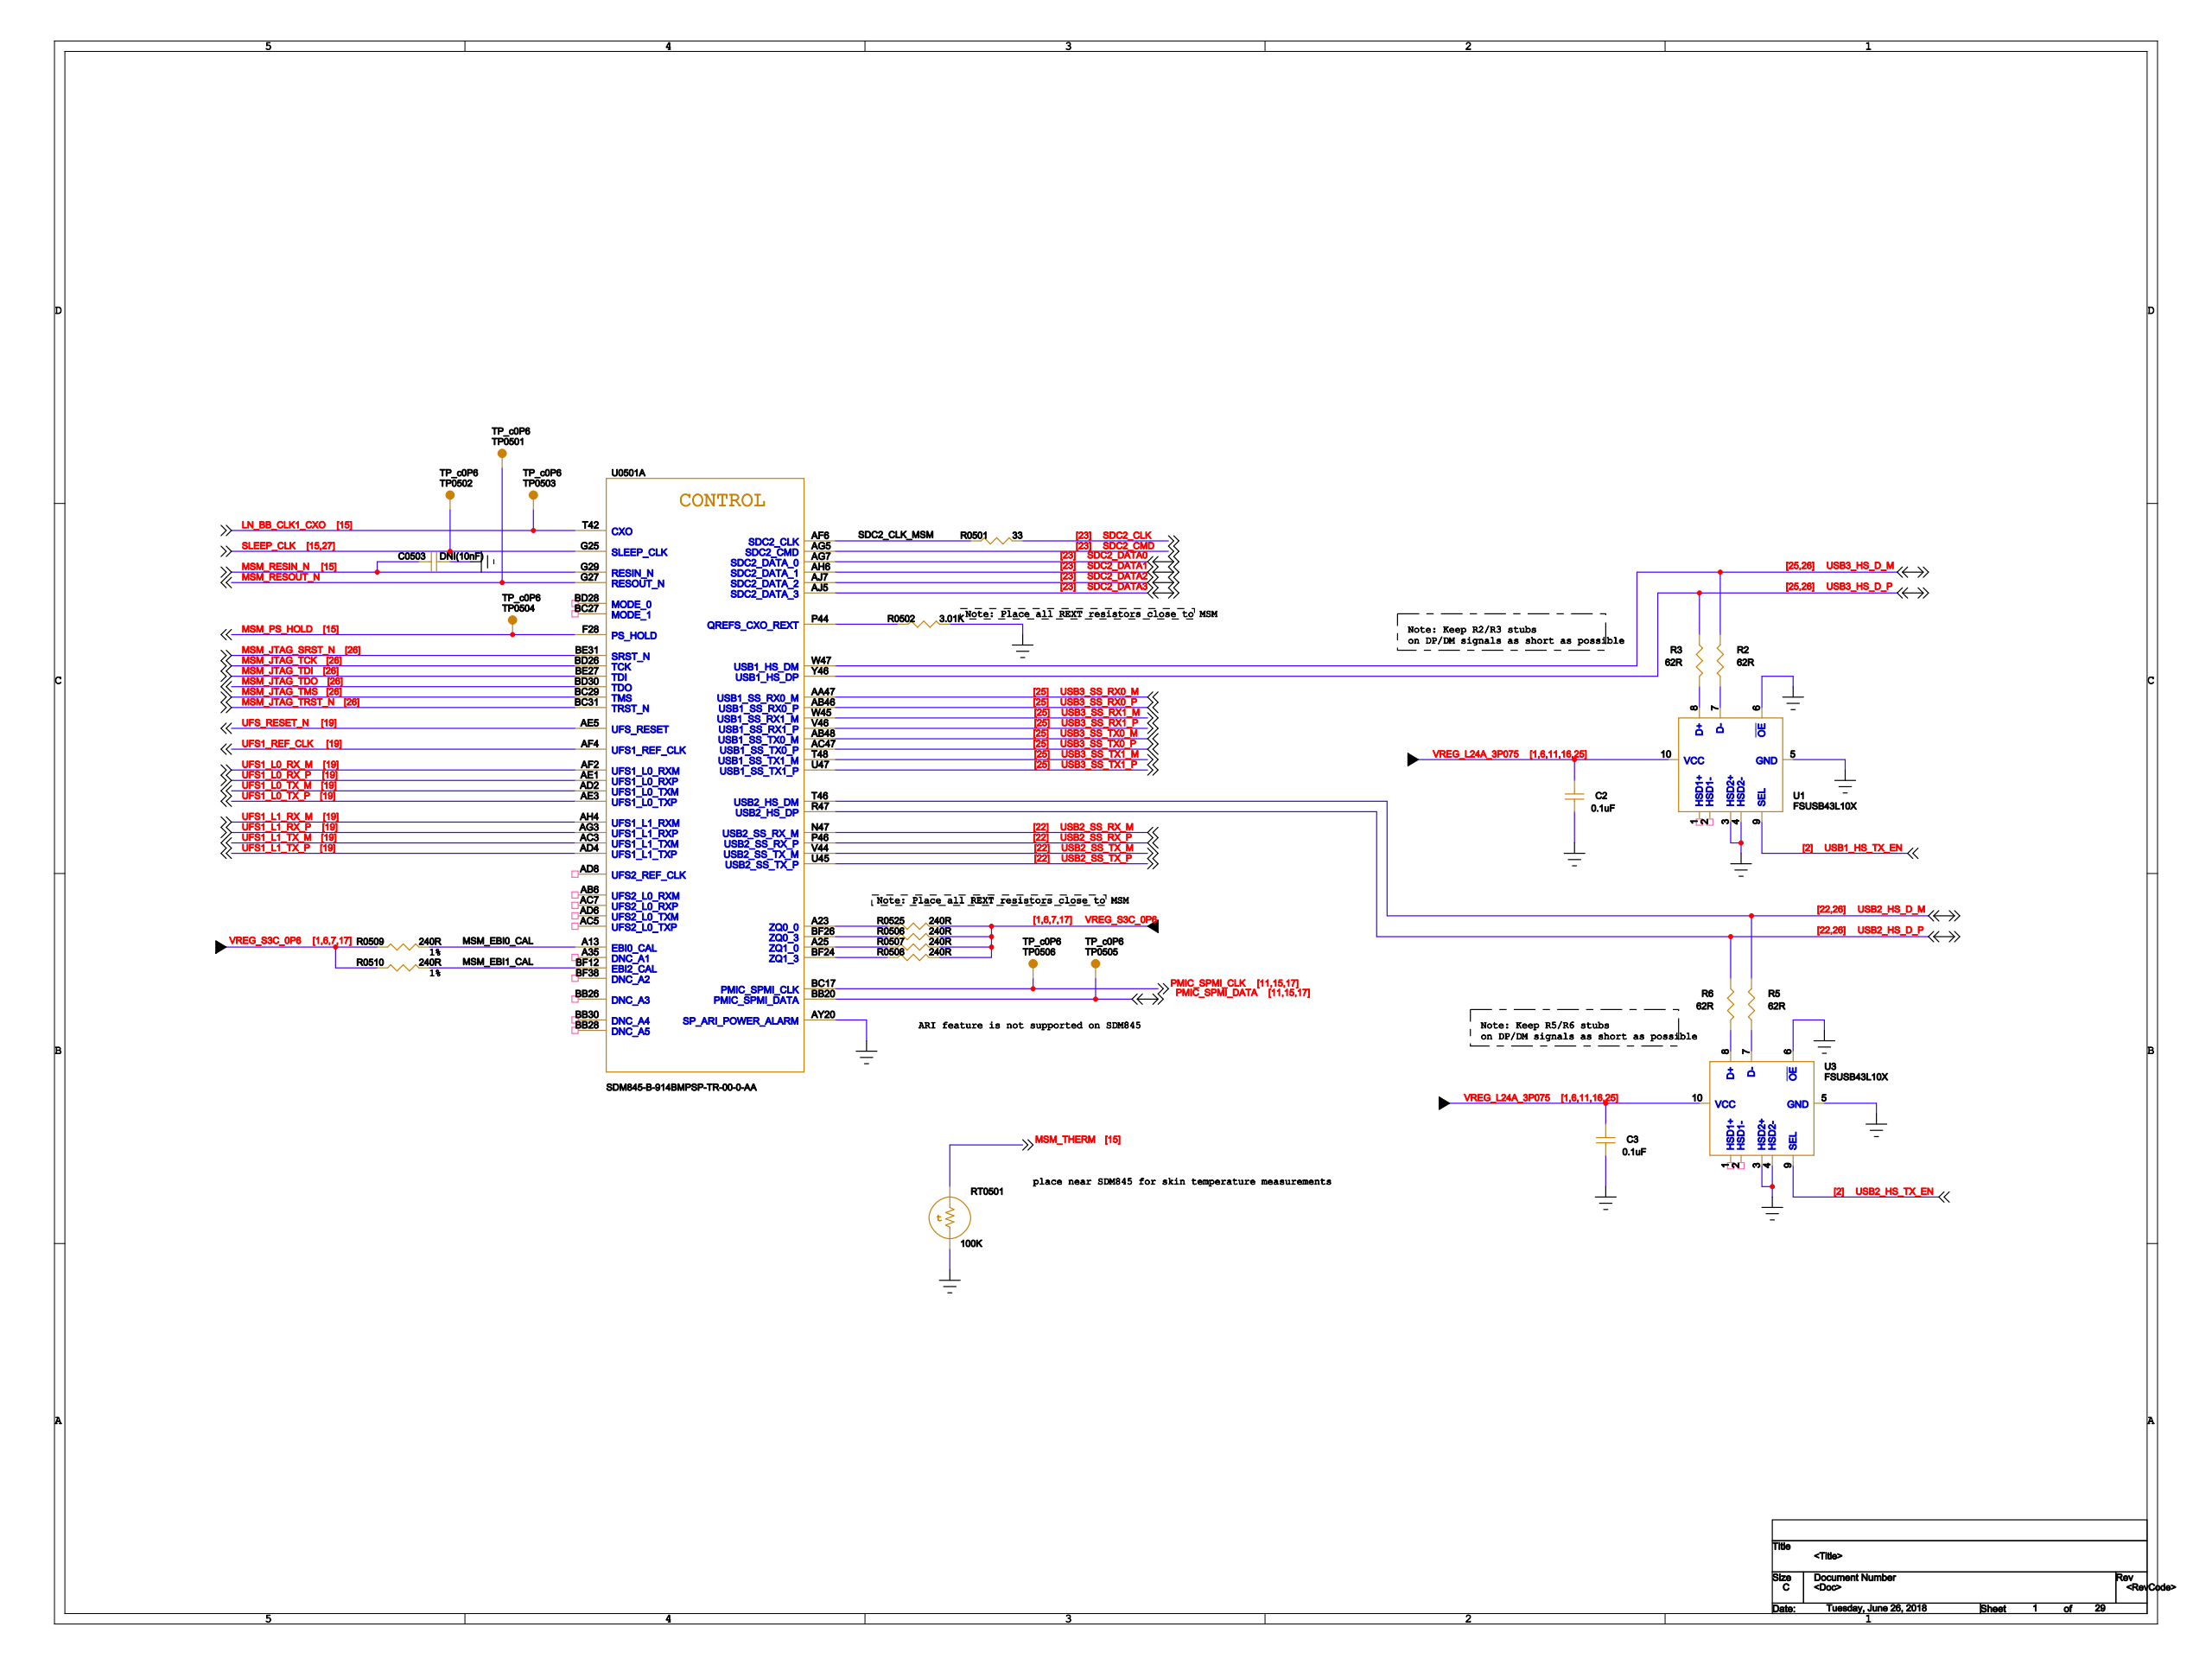Circuit board | Cadence Allegro | 802 parts | 566 nets | one sheet of the schematic
Parts on this sheet (reference | value | footprint):
C2 | 0.1uF | C0402
C3 | 0.1uF | C0402
C0503 | DNI(10nF) | C0201
R2 | 62R | R0201
R3 | 62R | R0201
R5 | 62R | R0201
R6 | 62R | R0201
R0501 | 33 | R0201
R0502 | 3.01K | R0402
R0506 | 240R | R0201
R0507 | 240R | R0201
R0508 | 240R | R0201
R0509 | 240R | R0201
R0510 | 240R | R0201
R0525 | 240R | R0201
RT0501 | 100K | R0402
TP0501 | TP_c0P6 | TP_C0P6
TP0502 | TP_c0P6 | TP_C0P6
TP0503 | TP_c0P6 | TP_C0P6
TP0504 | TP_c0P6 | TP_C0P6
TP0505 | TP_c0P6 | TP_C0P6
TP0506 | TP_c0P6 | TP_C0P6
U1 | FSUSB43L10X | UQFN10_1P6X2P1X0P5_0P65
U3 | FSUSB43L10X | UQFN10_1P6X2P1X0P5_0P65
U0501 | SDM845-B-914BMPSP-TR-00-0-AA | BGA914_12P4X12P4_0P58_0P35
Nets of these parts (net: part-pin ...):
MSM_RESIN_N: C0503-1 U0501-G29
GND: C2-1 C3-1 C0503-2 R0502-2 RT0501-2 U1-3 U1-4 U1-5 U1-6 U3-3 U3-4 U3-5 U3-6 U0501-AY20 U0501-C3 U0501-R5
VREG_L24A_3P075: C2-2 C3-2 U1-10 U3-10
SDC2_DATA3: U0501-AJ5
SDC2_DATA1: U0501-AH6
SDC2_CMD: U0501-AG5
SDC2_CLK: R0501-2
SDC2_DATA0: U0501-AG7
SDC2_DATA2: U0501-AJ7
USB3_SS_TX0_M: U0501-AB48
USB3_SS_TX0_P: U0501-AC47
USB3_SS_TX1_P: U0501-U47
USB3_SS_TX1_M: U0501-T48
VREG_S3C_0P6: R0506-2 R0507-2 R0508-2 R0509-1 R0510-1 R0525-2
USB3_HS_D_P: R3-2 U0501-Y46
USB3_HS_D_M: R2-2 U0501-W47
USB2_HS_D_P: R6-2 U0501-R47
USB2_HS_D_M: R5-2 U0501-T46
MSM_JTAG_SRST_N: U0501-BE31
MSM_JTAG_TRST_N: U0501-BC31
USB3_SS_RX0_M: U0501-AA47
USB3_SS_RX0_P: U0501-AB46
USB3_SS_RX1_P: U0501-V46
USB3_SS_RX1_M: U0501-W45
SDC2_CLK_MSM: R0501-1 U0501-AF6
N49611: R0502-1 U0501-P44
N50836: R0506-1 U0501-BF26
N50832: R0507-1 U0501-A25
N50828: R0508-1 U0501-BF24
MSM_EBI0_CAL: R0509-2 U0501-A13
MSM_EBI1_CAL: R0510-2 U0501-BF12
N50840: R0525-1 U0501-A23
N425370: R2-1 U1-7
N425398: R3-1 U1-8
N424667: R5-1 U3-7
N424700: R6-1 U3-8
MSM_THERM: RT0501-1
MSM_RESOUT_N: TP0501-1 U0501-G27
SLEEP_CLK: TP0502-1 U0501-G25
LN_BB_CLK1_CXO: TP0503-1 U0501-T42
MSM_PS_HOLD: TP0504-1 U0501-F28
PMIC_SPMI_DATA: TP0505-1 U0501-BB20
PMIC_SPMI_CLK: TP0506-1 U0501-BC17
UFS1_L0_RX_P: U0501-AE1
UFS1_L0_TX_M: U0501-AD2
UFS1_L0_TX_P: U0501-AE3
UFS1_L0_RX_M: U0501-AF2
MSM_JTAG_TDI: U0501-BE27
MSM_JTAG_TDO: U0501-BD30
MSM_JTAG_TCK: U0501-BD26
MSM_JTAG_TMS: U0501-BC29
UFS1_L1_RX_M: U0501-AH4
UFS1_L1_RX_P: U0501-AG3
UFS1_L1_TX_M: U0501-AC3
UFS1_L1_TX_P: U0501-AD4
UFS1_REF_CLK: U0501-AF4
UFS_RESET_N: U0501-AE5
USB2_SS_RX_M: U0501-N47
USB2_SS_RX_P: U0501-P46
USB2_SS_TX_M: U0501-V44
USB2_SS_TX_P: U0501-U45
USB1_HS_TX_EN: U1-9
USB2_HS_TX_EN: U3-9